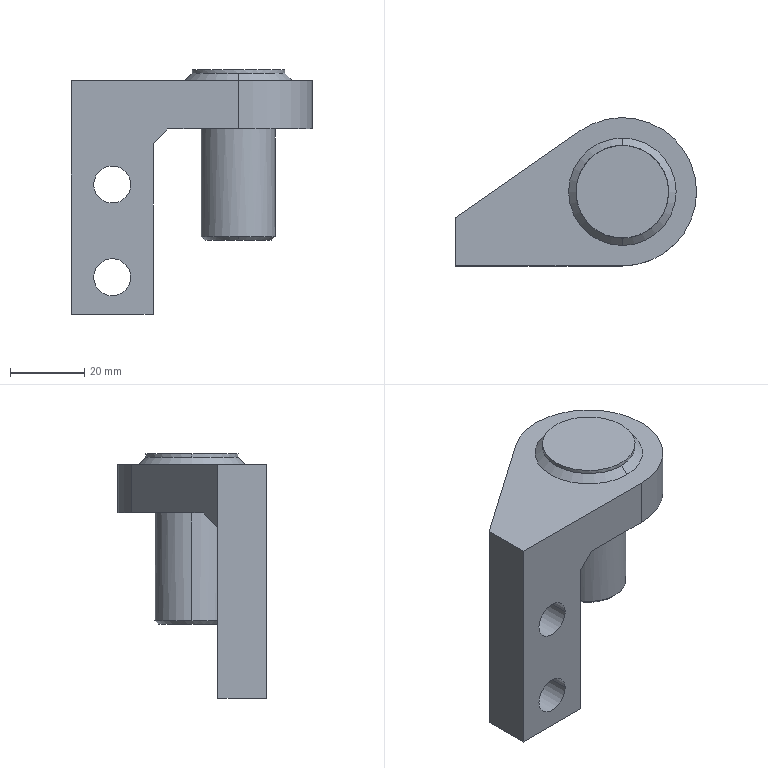Part | SolidWorks | features BaseBody 1 | 1 solid | 26 faces | box 65 x 40 x 66 mm | volume 48299 mm3 | plane 12 | cylinder 10 | cone 4 | commonest cylinder face diameters 10 x4 20 x2 25 x2 40 x2
STEP:
#1=CARTESIAN_POINT('',(14.621,16.327,0.));
#2=VERTEX_POINT('',#1);
#3=CARTESIAN_POINT('',(34.621,16.327,0.));
#4=VERTEX_POINT('',#3);
#5=CARTESIAN_POINT('',(24.621,16.327,0.));
#6=DIRECTION('',(0.,0.,-1.));
#7=DIRECTION('',(-1.,0.,0.));
#8=AXIS2_PLACEMENT_3D('',#5,#6,#7);
#9=CIRCLE('',#8,10.);
#10=EDGE_CURVE('',#2,#4,#9,.T.);
#11=ORIENTED_EDGE('',*,*,#10,.T.);
#12=CARTESIAN_POINT('',(34.621,16.327,-29.));
#13=VERTEX_POINT('',#12);
#14=CARTESIAN_POINT('',(34.621,16.327,0.));
#15=DIRECTION('',(0.,0.,-1.));
#16=VECTOR('',#15,1000.);
#17=LINE('',#14,#16);
#18=EDGE_CURVE('',#4,#13,#17,.T.);
#19=ORIENTED_EDGE('',*,*,#18,.T.);
#20=CARTESIAN_POINT('',(24.621,26.327,-29.));
#21=VERTEX_POINT('',#20);
#22=CARTESIAN_POINT('',(24.621,16.327,-29.));
#23=DIRECTION('',(0.,0.,1.));
#24=DIRECTION('',(-1.,0.,0.));
#25=AXIS2_PLACEMENT_3D('',#22,#23,#24);
#26=CIRCLE('',#25,10.);
#27=EDGE_CURVE('',#13,#21,#26,.T.);
#28=ORIENTED_EDGE('',*,*,#27,.T.);
#29=CARTESIAN_POINT('',(14.621,16.327,-29.));
#30=VERTEX_POINT('',#29);
#31=CARTESIAN_POINT('',(24.621,16.327,-29.));
#32=DIRECTION('',(0.,0.,1.));
#33=DIRECTION('',(-1.,0.,0.));
#34=AXIS2_PLACEMENT_3D('',#31,#32,#33);
#35=CIRCLE('',#34,10.);
#36=EDGE_CURVE('',#21,#30,#35,.T.);
#37=ORIENTED_EDGE('',*,*,#36,.T.);
#38=CARTESIAN_POINT('',(14.621,16.327,0.));
#39=DIRECTION('',(0.,0.,-1.));
#40=VECTOR('',#39,1000.);
#41=LINE('',#38,#40);
#42=EDGE_CURVE('',#2,#30,#41,.T.);
#43=ORIENTED_EDGE('',*,*,#42,.F.);
#44=EDGE_LOOP('',(#11,#19,#28,#37,#43));
#45=FACE_OUTER_BOUND('',#44,.T.);
#46=CARTESIAN_POINT('',(24.621,16.327,0.));
#47=DIRECTION('',(0.,0.,-1.));
#48=DIRECTION('',(-1.,0.,0.));
#49=AXIS2_PLACEMENT_3D('',#46,#47,#48);
#50=CYLINDRICAL_SURFACE('',#49,10.);
#51=ADVANCED_FACE('',(#45),#50,.T.);
#52=CARTESIAN_POINT('',(24.621,7.327,-30.));
#53=VERTEX_POINT('',#52);
#54=CARTESIAN_POINT('',(24.621,25.327,-30.));
#55=VERTEX_POINT('',#54);
#56=CARTESIAN_POINT('',(24.621,16.327,-30.));
#57=DIRECTION('',(0.,0.,1.));
#58=DIRECTION('',(0.,-1.,0.));
#59=AXIS2_PLACEMENT_3D('',#56,#57,#58);
#60=CIRCLE('',#59,9.);
#61=EDGE_CURVE('',#53,#55,#60,.T.);
#62=ORIENTED_EDGE('',*,*,#61,.T.);
#63=CARTESIAN_POINT('',(24.621,26.327,-29.));
#64=DIRECTION('',(0.,0.7071,0.7071));
#65=VECTOR('',#64,1000.);
#66=LINE('',#63,#65);
#67=EDGE_CURVE('',#55,#21,#66,.T.);
#68=ORIENTED_EDGE('',*,*,#67,.T.);
#69=ORIENTED_EDGE('',*,*,#27,.F.);
#70=CARTESIAN_POINT('',(24.621,6.327,-29.));
#71=VERTEX_POINT('',#70);
#72=CARTESIAN_POINT('',(24.621,16.327,-29.));
#73=DIRECTION('',(0.,0.,1.));
#74=DIRECTION('',(-1.,0.,0.));
#75=AXIS2_PLACEMENT_3D('',#72,#73,#74);
#76=CIRCLE('',#75,10.);
#77=EDGE_CURVE('',#71,#13,#76,.T.);
#78=ORIENTED_EDGE('',*,*,#77,.F.);
#79=CARTESIAN_POINT('',(24.621,6.327,-29.));
#80=DIRECTION('',(0.,-0.7071,0.7071));
#81=VECTOR('',#80,1000.);
#82=LINE('',#79,#81);
#83=EDGE_CURVE('',#53,#71,#82,.T.);
#84=ORIENTED_EDGE('',*,*,#83,.F.);
#85=EDGE_LOOP('',(#62,#68,#69,#78,#84));
#86=FACE_OUTER_BOUND('',#85,.T.);
#87=CARTESIAN_POINT('',(24.621,16.327,-29.));
#88=DIRECTION('',(0.,0.,1.));
#89=DIRECTION('',(0.,-1.,0.));
#90=AXIS2_PLACEMENT_3D('',#87,#88,#89);
#91=CONICAL_SURFACE('',#90,10.,0.7854);
#92=ADVANCED_FACE('',(#86),#91,.T.);
#93=CARTESIAN_POINT('',(24.621,-3.673,0.));
#94=VERTEX_POINT('',#93);
#95=CARTESIAN_POINT('',(44.621,16.327,0.));
#96=VERTEX_POINT('',#95);
#97=CARTESIAN_POINT('',(24.621,16.327,0.));
#98=DIRECTION('',(0.,0.,1.));
#99=DIRECTION('',(1.,0.,0.));
#100=AXIS2_PLACEMENT_3D('',#97,#98,#99);
#101=CIRCLE('',#100,20.);
#102=EDGE_CURVE('',#94,#96,#101,.T.);
#103=ORIENTED_EDGE('',*,*,#102,.T.);
#104=CARTESIAN_POINT('',(44.621,16.327,13.));
#105=VERTEX_POINT('',#104);
#106=CARTESIAN_POINT('',(44.621,16.327,0.));
#107=DIRECTION('',(0.,0.,1.));
#108=VECTOR('',#107,1000.);
#109=LINE('',#106,#108);
#110=EDGE_CURVE('',#96,#105,#109,.T.);
#111=ORIENTED_EDGE('',*,*,#110,.T.);
#112=CARTESIAN_POINT('',(24.621,-3.673,13.));
#113=VERTEX_POINT('',#112);
#114=CARTESIAN_POINT('',(24.621,16.327,13.));
#115=DIRECTION('',(0.,0.,-1.));
#116=DIRECTION('',(1.,0.,0.));
#117=AXIS2_PLACEMENT_3D('',#114,#115,#116);
#118=CIRCLE('',#117,20.);
#119=EDGE_CURVE('',#105,#113,#118,.T.);
#120=ORIENTED_EDGE('',*,*,#119,.T.);
#121=CARTESIAN_POINT('',(24.621,-3.673,0.));
#122=DIRECTION('',(0.,0.,-1.));
#123=VECTOR('',#122,1000.);
#124=LINE('',#121,#123);
#125=EDGE_CURVE('',#113,#94,#124,.T.);
#126=ORIENTED_EDGE('',*,*,#125,.T.);
#127=EDGE_LOOP('',(#103,#111,#120,#126));
#128=FACE_OUTER_BOUND('',#127,.T.);
#129=CARTESIAN_POINT('',(24.621,16.327,0.));
#130=DIRECTION('',(0.,0.,1.));
#131=DIRECTION('',(1.,0.,0.));
#132=AXIS2_PLACEMENT_3D('',#129,#130,#131);
#133=CYLINDRICAL_SURFACE('',#132,20.);
#134=ADVANCED_FACE('',(#128),#133,.T.);
#135=CARTESIAN_POINT('',(-4.379,-3.673,-40.));
#136=VERTEX_POINT('',#135);
#137=CARTESIAN_POINT('',(-14.379,-3.673,-40.));
#138=VERTEX_POINT('',#137);
#139=CARTESIAN_POINT('',(-9.379,-3.673,-40.));
#140=DIRECTION('',(0.,1.,0.));
#141=DIRECTION('',(-1.,0.,0.));
#142=AXIS2_PLACEMENT_3D('',#139,#140,#141);
#143=CIRCLE('',#142,5.);
#144=EDGE_CURVE('',#136,#138,#143,.T.);
#145=ORIENTED_EDGE('',*,*,#144,.F.);
#146=CARTESIAN_POINT('',(-4.379,9.327,-40.));
#147=VERTEX_POINT('',#146);
#148=CARTESIAN_POINT('',(-4.379,-91.574,-40.));
#149=DIRECTION('',(0.,1.,0.));
#150=VECTOR('',#149,1000.);
#151=LINE('',#148,#150);
#152=EDGE_CURVE('',#136,#147,#151,.T.);
#153=ORIENTED_EDGE('',*,*,#152,.T.);
#154=CARTESIAN_POINT('',(-14.379,9.327,-40.));
#155=VERTEX_POINT('',#154);
#156=CARTESIAN_POINT('',(-9.379,9.327,-40.));
#157=DIRECTION('',(0.,-1.,0.));
#158=DIRECTION('',(-1.,0.,0.));
#159=AXIS2_PLACEMENT_3D('',#156,#157,#158);
#160=CIRCLE('',#159,5.);
#161=EDGE_CURVE('',#155,#147,#160,.T.);
#162=ORIENTED_EDGE('',*,*,#161,.F.);
#163=CARTESIAN_POINT('',(-14.379,-91.574,-40.));
#164=DIRECTION('',(0.,1.,0.));
#165=VECTOR('',#164,1000.);
#166=LINE('',#163,#165);
#167=EDGE_CURVE('',#138,#155,#166,.T.);
#168=ORIENTED_EDGE('',*,*,#167,.F.);
#169=EDGE_LOOP('',(#145,#153,#162,#168));
#170=FACE_OUTER_BOUND('',#169,.T.);
#171=CARTESIAN_POINT('',(-9.379,-91.574,-40.));
#172=DIRECTION('',(0.,1.,0.));
#173=DIRECTION('',(-1.,0.,0.));
#174=AXIS2_PLACEMENT_3D('',#171,#172,#173);
#175=CYLINDRICAL_SURFACE('',#174,5.);
#176=ADVANCED_FACE('',(#170),#175,.F.);
#177=CARTESIAN_POINT('',(-4.379,-3.673,-15.));
#178=VERTEX_POINT('',#177);
#179=CARTESIAN_POINT('',(-14.379,-3.673,-15.));
#180=VERTEX_POINT('',#179);
#181=CARTESIAN_POINT('',(-9.379,-3.673,-15.));
#182=DIRECTION('',(0.,1.,0.));
#183=DIRECTION('',(-1.,0.,0.));
#184=AXIS2_PLACEMENT_3D('',#181,#182,#183);
#185=CIRCLE('',#184,5.);
#186=EDGE_CURVE('',#178,#180,#185,.T.);
#187=ORIENTED_EDGE('',*,*,#186,.F.);
#188=CARTESIAN_POINT('',(-4.379,9.327,-15.));
#189=VERTEX_POINT('',#188);
#190=CARTESIAN_POINT('',(-4.379,-91.574,-15.));
#191=DIRECTION('',(0.,1.,0.));
#192=VECTOR('',#191,1000.);
#193=LINE('',#190,#192);
#194=EDGE_CURVE('',#178,#189,#193,.T.);
#195=ORIENTED_EDGE('',*,*,#194,.T.);
#196=CARTESIAN_POINT('',(-14.379,9.327,-15.));
#197=VERTEX_POINT('',#196);
#198=CARTESIAN_POINT('',(-9.379,9.327,-15.));
#199=DIRECTION('',(0.,-1.,0.));
#200=DIRECTION('',(-1.,0.,0.));
#201=AXIS2_PLACEMENT_3D('',#198,#199,#200);
#202=CIRCLE('',#201,5.);
#203=EDGE_CURVE('',#197,#189,#202,.T.);
#204=ORIENTED_EDGE('',*,*,#203,.F.);
#205=CARTESIAN_POINT('',(-14.379,-91.574,-15.));
#206=DIRECTION('',(0.,1.,0.));
#207=VECTOR('',#206,1000.);
#208=LINE('',#205,#207);
#209=EDGE_CURVE('',#180,#197,#208,.T.);
#210=ORIENTED_EDGE('',*,*,#209,.F.);
#211=EDGE_LOOP('',(#187,#195,#204,#210));
#212=FACE_OUTER_BOUND('',#211,.T.);
#213=CARTESIAN_POINT('',(-9.379,-91.574,-15.));
#214=DIRECTION('',(0.,1.,0.));
#215=DIRECTION('',(-1.,0.,0.));
#216=AXIS2_PLACEMENT_3D('',#213,#214,#215);
#217=CYLINDRICAL_SURFACE('',#216,5.);
#218=ADVANCED_FACE('',(#212),#217,.F.);
#219=CARTESIAN_POINT('',(37.121,16.327,15.));
#220=VERTEX_POINT('',#219);
#221=CARTESIAN_POINT('',(24.621,3.827,15.));
#222=VERTEX_POINT('',#221);
#223=CARTESIAN_POINT('',(24.621,16.327,15.));
#224=DIRECTION('',(0.,0.,-1.));
#225=DIRECTION('',(-1.,0.,0.));
#226=AXIS2_PLACEMENT_3D('',#223,#224,#225);
#227=CIRCLE('',#226,12.5);
#228=EDGE_CURVE('',#220,#222,#227,.T.);
#229=ORIENTED_EDGE('',*,*,#228,.T.);
#230=CARTESIAN_POINT('',(24.621,1.827,13.));
#231=VERTEX_POINT('',#230);
#232=CARTESIAN_POINT('',(24.621,1.827,13.));
#233=DIRECTION('',(0.,-0.7071,-0.7071));
#234=VECTOR('',#233,1000.);
#235=LINE('',#232,#234);
#236=EDGE_CURVE('',#222,#231,#235,.T.);
#237=ORIENTED_EDGE('',*,*,#236,.T.);
#238=CARTESIAN_POINT('',(24.621,30.827,13.));
#239=VERTEX_POINT('',#238);
#240=CARTESIAN_POINT('',(24.621,16.327,13.));
#241=DIRECTION('',(0.,0.,-1.));
#242=DIRECTION('',(0.,1.,0.));
#243=AXIS2_PLACEMENT_3D('',#240,#241,#242);
#244=CIRCLE('',#243,14.5);
#245=EDGE_CURVE('',#239,#231,#244,.T.);
#246=ORIENTED_EDGE('',*,*,#245,.F.);
#247=CARTESIAN_POINT('',(24.621,28.827,15.));
#248=VERTEX_POINT('',#247);
#249=CARTESIAN_POINT('',(24.621,30.827,13.));
#250=DIRECTION('',(0.,0.7071,-0.7071));
#251=VECTOR('',#250,1000.);
#252=LINE('',#249,#251);
#253=EDGE_CURVE('',#248,#239,#252,.T.);
#254=ORIENTED_EDGE('',*,*,#253,.F.);
#255=CARTESIAN_POINT('',(24.621,16.327,15.));
#256=DIRECTION('',(0.,0.,-1.));
#257=DIRECTION('',(-1.,0.,0.));
#258=AXIS2_PLACEMENT_3D('',#255,#256,#257);
#259=CIRCLE('',#258,12.5);
#260=EDGE_CURVE('',#248,#220,#259,.T.);
#261=ORIENTED_EDGE('',*,*,#260,.T.);
#262=EDGE_LOOP('',(#229,#237,#246,#254,#261));
#263=FACE_OUTER_BOUND('',#262,.T.);
#264=CARTESIAN_POINT('',(24.621,16.327,13.));
#265=DIRECTION('',(0.,0.,-1.));
#266=DIRECTION('',(0.,1.,0.));
#267=AXIS2_PLACEMENT_3D('',#264,#265,#266);
#268=CONICAL_SURFACE('',#267,14.5,0.7854);
#269=ADVANCED_FACE('',(#263),#268,.T.);
#270=CARTESIAN_POINT('',(12.121,16.327,15.));
#271=VERTEX_POINT('',#270);
#272=CARTESIAN_POINT('',(24.621,16.327,15.));
#273=DIRECTION('',(0.,0.,-1.));
#274=DIRECTION('',(-1.,0.,0.));
#275=AXIS2_PLACEMENT_3D('',#272,#273,#274);
#276=CIRCLE('',#275,12.5);
#277=EDGE_CURVE('',#271,#248,#276,.T.);
#278=ORIENTED_EDGE('',*,*,#277,.F.);
#279=CARTESIAN_POINT('',(12.121,16.327,16.));
#280=VERTEX_POINT('',#279);
#281=CARTESIAN_POINT('',(12.121,16.327,13.));
#282=DIRECTION('',(0.,0.,1.));
#283=VECTOR('',#282,1000.);
#284=LINE('',#281,#283);
#285=EDGE_CURVE('',#271,#280,#284,.T.);
#286=ORIENTED_EDGE('',*,*,#285,.T.);
#287=CARTESIAN_POINT('',(37.121,16.327,16.));
#288=VERTEX_POINT('',#287);
#289=CARTESIAN_POINT('',(24.621,16.327,16.));
#290=DIRECTION('',(0.,0.,-1.));
#291=DIRECTION('',(1.,0.,0.));
#292=AXIS2_PLACEMENT_3D('',#289,#290,#291);
#293=CIRCLE('',#292,12.5);
#294=EDGE_CURVE('',#280,#288,#293,.T.);
#295=ORIENTED_EDGE('',*,*,#294,.T.);
#296=CARTESIAN_POINT('',(37.121,16.327,13.));
#297=DIRECTION('',(0.,0.,1.));
#298=VECTOR('',#297,1000.);
#299=LINE('',#296,#298);
#300=EDGE_CURVE('',#220,#288,#299,.T.);
#301=ORIENTED_EDGE('',*,*,#300,.F.);
#302=ORIENTED_EDGE('',*,*,#260,.F.);
#303=EDGE_LOOP('',(#278,#286,#295,#301,#302));
#304=FACE_OUTER_BOUND('',#303,.T.);
#305=CARTESIAN_POINT('',(24.621,16.327,13.));
#306=DIRECTION('',(0.,0.,1.));
#307=DIRECTION('',(1.,0.,0.));
#308=AXIS2_PLACEMENT_3D('',#305,#306,#307);
#309=CYLINDRICAL_SURFACE('',#308,12.5);
#310=ADVANCED_FACE('',(#304),#309,.T.);
#311=ORIENTED_EDGE('',*,*,#18,.F.);
#312=CARTESIAN_POINT('',(24.621,16.327,0.));
#313=DIRECTION('',(0.,0.,-1.));
#314=DIRECTION('',(-1.,0.,0.));
#315=AXIS2_PLACEMENT_3D('',#312,#313,#314);
#316=CIRCLE('',#315,10.);
#317=EDGE_CURVE('',#4,#2,#316,.T.);
#318=ORIENTED_EDGE('',*,*,#317,.T.);
#319=ORIENTED_EDGE('',*,*,#42,.T.);
#320=CARTESIAN_POINT('',(24.621,16.327,-29.));
#321=DIRECTION('',(0.,0.,1.));
#322=DIRECTION('',(-1.,0.,0.));
#323=AXIS2_PLACEMENT_3D('',#320,#321,#322);
#324=CIRCLE('',#323,10.);
#325=EDGE_CURVE('',#30,#71,#324,.T.);
#326=ORIENTED_EDGE('',*,*,#325,.T.);
#327=ORIENTED_EDGE('',*,*,#77,.T.);
#328=EDGE_LOOP('',(#311,#318,#319,#326,#327));
#329=FACE_OUTER_BOUND('',#328,.T.);
#330=CARTESIAN_POINT('',(24.621,16.327,0.));
#331=DIRECTION('',(0.,0.,-1.));
#332=DIRECTION('',(-1.,0.,0.));
#333=AXIS2_PLACEMENT_3D('',#330,#331,#332);
#334=CYLINDRICAL_SURFACE('',#333,10.);
#335=ADVANCED_FACE('',(#329),#334,.T.);
#336=ORIENTED_EDGE('',*,*,#67,.F.);
#337=CARTESIAN_POINT('',(24.621,16.327,-30.));
#338=DIRECTION('',(0.,0.,1.));
#339=DIRECTION('',(0.,-1.,0.));
#340=AXIS2_PLACEMENT_3D('',#337,#338,#339);
#341=CIRCLE('',#340,9.);
#342=EDGE_CURVE('',#55,#53,#341,.T.);
#343=ORIENTED_EDGE('',*,*,#342,.T.);
#344=ORIENTED_EDGE('',*,*,#83,.T.);
#345=ORIENTED_EDGE('',*,*,#325,.F.);
#346=ORIENTED_EDGE('',*,*,#36,.F.);
#347=EDGE_LOOP('',(#336,#343,#344,#345,#346));
#348=FACE_OUTER_BOUND('',#347,.T.);
#349=CARTESIAN_POINT('',(24.621,16.327,-29.));
#350=DIRECTION('',(0.,0.,1.));
#351=DIRECTION('',(0.,-1.,0.));
#352=AXIS2_PLACEMENT_3D('',#349,#350,#351);
#353=CONICAL_SURFACE('',#352,10.,0.7854);
#354=ADVANCED_FACE('',(#348),#353,.T.);
#355=ORIENTED_EDGE('',*,*,#10,.F.);
#356=ORIENTED_EDGE('',*,*,#317,.F.);
#357=EDGE_LOOP('',(#355,#356));
#358=FACE_BOUND('',#357,.T.);
#359=CARTESIAN_POINT('',(-14.644,13.327,0.));
#360=VERTEX_POINT('',#359);
#361=CARTESIAN_POINT('',(5.621,13.327,0.));
#362=VERTEX_POINT('',#361);
#363=CARTESIAN_POINT('',(12.334,13.327,0.));
#364=DIRECTION('',(1.,0.,0.));
#365=VECTOR('',#364,1000.);
#366=LINE('',#363,#365);
#367=EDGE_CURVE('',#360,#362,#366,.T.);
#368=ORIENTED_EDGE('',*,*,#367,.F.);
#369=CARTESIAN_POINT('',(13.18,32.732,0.));
#370=VERTEX_POINT('',#369);
#371=CARTESIAN_POINT('',(13.18,32.732,0.));
#372=DIRECTION('',(-0.8202,-0.572,0.));
#373=VECTOR('',#372,1000.);
#374=LINE('',#371,#373);
#375=EDGE_CURVE('',#370,#360,#374,.T.);
#376=ORIENTED_EDGE('',*,*,#375,.F.);
#377=CARTESIAN_POINT('',(24.621,16.327,0.));
#378=DIRECTION('',(0.,0.,1.));
#379=DIRECTION('',(1.,0.,0.));
#380=AXIS2_PLACEMENT_3D('',#377,#378,#379);
#381=CIRCLE('',#380,20.);
#382=EDGE_CURVE('',#96,#370,#381,.T.);
#383=ORIENTED_EDGE('',*,*,#382,.F.);
#384=ORIENTED_EDGE('',*,*,#102,.F.);
#385=CARTESIAN_POINT('',(5.621,-3.673,0.));
#386=VERTEX_POINT('',#385);
#387=CARTESIAN_POINT('',(12.334,-3.673,0.));
#388=DIRECTION('',(1.,0.,0.));
#389=VECTOR('',#388,1000.);
#390=LINE('',#387,#389);
#391=EDGE_CURVE('',#386,#94,#390,.T.);
#392=ORIENTED_EDGE('',*,*,#391,.F.);
#393=CARTESIAN_POINT('',(5.621,12.361,0.));
#394=DIRECTION('',(0.,-1.,0.));
#395=VECTOR('',#394,1000.);
#396=LINE('',#393,#395);
#397=EDGE_CURVE('',#362,#386,#396,.T.);
#398=ORIENTED_EDGE('',*,*,#397,.F.);
#399=EDGE_LOOP('',(#368,#376,#383,#384,#392,#398));
#400=FACE_OUTER_BOUND('',#399,.T.);
#401=CARTESIAN_POINT('',(12.334,12.361,0.));
#402=DIRECTION('',(0.,0.,1.));
#403=DIRECTION('',(1.,0.,0.));
#404=AXIS2_PLACEMENT_3D('',#401,#402,#403);
#405=PLANE('',#404);
#406=ADVANCED_FACE('',(#358,#400),#405,.F.);
#407=ORIENTED_EDGE('',*,*,#61,.F.);
#408=ORIENTED_EDGE('',*,*,#342,.F.);
#409=EDGE_LOOP('',(#407,#408));
#410=FACE_OUTER_BOUND('',#409,.T.);
#411=CARTESIAN_POINT('',(24.621,16.327,-30.));
#412=DIRECTION('',(0.,0.,1.));
#413=DIRECTION('',(1.,0.,0.));
#414=AXIS2_PLACEMENT_3D('',#411,#412,#413);
#415=PLANE('',#414);
#416=ADVANCED_FACE('',(#410),#415,.F.);
#417=CARTESIAN_POINT('',(1.621,9.327,-4.));
#418=VERTEX_POINT('',#417);
#419=CARTESIAN_POINT('',(1.621,9.327,-4.));
#420=DIRECTION('',(0.5774,0.5774,0.5774));
#421=VECTOR('',#420,1000.);
#422=LINE('',#419,#421);
#423=EDGE_CURVE('',#418,#362,#422,.T.);
#424=ORIENTED_EDGE('',*,*,#423,.T.);
#425=ORIENTED_EDGE('',*,*,#397,.T.);
#426=CARTESIAN_POINT('',(1.621,-3.673,-4.));
#427=VERTEX_POINT('',#426);
#428=CARTESIAN_POINT('',(3.621,-3.673,-2.));
#429=DIRECTION('',(-0.7071,0.,-0.7071));
#430=VECTOR('',#429,1000.);
#431=LINE('',#428,#430);
#432=EDGE_CURVE('',#386,#427,#431,.T.);
#433=ORIENTED_EDGE('',*,*,#432,.T.);
#434=CARTESIAN_POINT('',(1.621,4.344,-4.));
#435=DIRECTION('',(0.,1.,0.));
#436=VECTOR('',#435,1000.);
#437=LINE('',#434,#436);
#438=EDGE_CURVE('',#427,#418,#437,.T.);
#439=ORIENTED_EDGE('',*,*,#438,.T.);
#440=EDGE_LOOP('',(#424,#425,#433,#439));
#441=FACE_OUTER_BOUND('',#440,.T.);
#442=CARTESIAN_POINT('',(3.621,4.344,-2.));
#443=DIRECTION('',(0.7071,0.,-0.7071));
#444=DIRECTION('',(-0.7071,0.,-0.7071));
#445=AXIS2_PLACEMENT_3D('',#442,#443,#444);
#446=PLANE('',#445);
#447=ADVANCED_FACE('',(#441),#446,.T.);
#448=ORIENTED_EDGE('',*,*,#423,.F.);
#449=CARTESIAN_POINT('',(-20.379,9.327,-4.));
#450=VERTEX_POINT('',#449);
#451=CARTESIAN_POINT('',(6.977,9.327,-4.));
#452=DIRECTION('',(-1.,0.,0.));
#453=VECTOR('',#452,1000.);
#454=LINE('',#451,#453);
#455=EDGE_CURVE('',#418,#450,#454,.T.);
#456=ORIENTED_EDGE('',*,*,#455,.T.);
#457=CARTESIAN_POINT('',(-20.379,9.327,-4.));
#458=DIRECTION('',(0.712,0.4965,0.4965));
#459=VECTOR('',#458,1000.);
#460=LINE('',#457,#459);
#461=EDGE_CURVE('',#450,#360,#460,.T.);
#462=ORIENTED_EDGE('',*,*,#461,.T.);
#463=ORIENTED_EDGE('',*,*,#367,.T.);
#464=EDGE_LOOP('',(#448,#456,#462,#463));
#465=FACE_OUTER_BOUND('',#464,.T.);
#466=CARTESIAN_POINT('',(6.977,11.327,-2.));
#467=DIRECTION('',(0.,0.7071,-0.7071));
#468=DIRECTION('',(0.,0.7071,0.7071));
#469=AXIS2_PLACEMENT_3D('',#466,#467,#468);
#470=PLANE('',#469);
#471=ADVANCED_FACE('',(#465),#470,.T.);
#472=ORIENTED_EDGE('',*,*,#461,.F.);
#473=CARTESIAN_POINT('',(-20.379,9.327,13.));
#474=VERTEX_POINT('',#473);
#475=CARTESIAN_POINT('',(-20.379,9.327,0.));
#476=DIRECTION('',(0.,0.,1.));
#477=VECTOR('',#476,1000.);
#478=LINE('',#475,#477);
#479=EDGE_CURVE('',#450,#474,#478,.T.);
#480=ORIENTED_EDGE('',*,*,#479,.T.);
#481=CARTESIAN_POINT('',(13.18,32.732,13.));
#482=VERTEX_POINT('',#481);
#483=CARTESIAN_POINT('',(-20.379,9.327,13.));
#484=DIRECTION('',(0.8202,0.572,0.));
#485=VECTOR('',#484,1000.);
#486=LINE('',#483,#485);
#487=EDGE_CURVE('',#474,#482,#486,.T.);
#488=ORIENTED_EDGE('',*,*,#487,.T.);
#489=CARTESIAN_POINT('',(13.18,32.732,0.));
#490=DIRECTION('',(0.,0.,-1.));
#491=VECTOR('',#490,1000.);
#492=LINE('',#489,#491);
#493=EDGE_CURVE('',#482,#370,#492,.T.);
#494=ORIENTED_EDGE('',*,*,#493,.T.);
#495=ORIENTED_EDGE('',*,*,#375,.T.);
#496=EDGE_LOOP('',(#472,#480,#488,#494,#495));
#497=FACE_OUTER_BOUND('',#496,.T.);
#498=CARTESIAN_POINT('',(-20.379,9.327,0.));
#499=DIRECTION('',(-0.572,0.8202,0.));
#500=DIRECTION('',(-0.8202,-0.572,0.));
#501=AXIS2_PLACEMENT_3D('',#498,#499,#500);
#502=PLANE('',#501);
#503=ADVANCED_FACE('',(#497),#502,.T.);
#504=ORIENTED_EDGE('',*,*,#110,.F.);
#505=ORIENTED_EDGE('',*,*,#382,.T.);
#506=ORIENTED_EDGE('',*,*,#493,.F.);
#507=CARTESIAN_POINT('',(24.621,16.327,13.));
#508=DIRECTION('',(0.,0.,-1.));
#509=DIRECTION('',(1.,0.,0.));
#510=AXIS2_PLACEMENT_3D('',#507,#508,#509);
#511=CIRCLE('',#510,20.);
#512=EDGE_CURVE('',#482,#105,#511,.T.);
#513=ORIENTED_EDGE('',*,*,#512,.T.);
#514=EDGE_LOOP('',(#504,#505,#506,#513));
#515=FACE_OUTER_BOUND('',#514,.T.);
#516=CARTESIAN_POINT('',(24.621,16.327,0.));
#517=DIRECTION('',(0.,0.,1.));
#518=DIRECTION('',(1.,0.,0.));
#519=AXIS2_PLACEMENT_3D('',#516,#517,#518);
#520=CYLINDRICAL_SURFACE('',#519,20.);
#521=ADVANCED_FACE('',(#515),#520,.T.);
#522=CARTESIAN_POINT('',(-9.379,-3.673,-40.));
#523=DIRECTION('',(0.,1.,0.));
#524=DIRECTION('',(-1.,0.,0.));
#525=AXIS2_PLACEMENT_3D('',#522,#523,#524);
#526=CIRCLE('',#525,5.);
#527=EDGE_CURVE('',#138,#136,#526,.T.);
#528=ORIENTED_EDGE('',*,*,#527,.T.);
#529=ORIENTED_EDGE('',*,*,#144,.T.);
#530=EDGE_LOOP('',(#528,#529));
#531=FACE_BOUND('',#530,.T.);
#532=CARTESIAN_POINT('',(-9.379,-3.673,-15.));
#533=DIRECTION('',(0.,1.,0.));
#534=DIRECTION('',(-1.,0.,0.));
#535=AXIS2_PLACEMENT_3D('',#532,#533,#534);
#536=CIRCLE('',#535,5.);
#537=EDGE_CURVE('',#180,#178,#536,.T.);
#538=ORIENTED_EDGE('',*,*,#537,.T.);
#539=ORIENTED_EDGE('',*,*,#186,.T.);
#540=EDGE_LOOP('',(#538,#539));
#541=FACE_BOUND('',#540,.T.);
#542=ORIENTED_EDGE('',*,*,#391,.T.);
#543=ORIENTED_EDGE('',*,*,#125,.F.);
#544=CARTESIAN_POINT('',(-20.379,-3.673,13.));
#545=VERTEX_POINT('',#544);
#546=CARTESIAN_POINT('',(24.621,-3.673,13.));
#547=DIRECTION('',(-1.,0.,0.));
#548=VECTOR('',#547,1000.);
#549=LINE('',#546,#548);
#550=EDGE_CURVE('',#113,#545,#549,.T.);
#551=ORIENTED_EDGE('',*,*,#550,.T.);
#552=CARTESIAN_POINT('',(-20.379,-3.673,-50.));
#553=VERTEX_POINT('',#552);
#554=CARTESIAN_POINT('',(-20.379,-3.673,0.));
#555=DIRECTION('',(0.,0.,-1.));
#556=VECTOR('',#555,1000.);
#557=LINE('',#554,#556);
#558=EDGE_CURVE('',#545,#553,#557,.T.);
#559=ORIENTED_EDGE('',*,*,#558,.T.);
#560=CARTESIAN_POINT('',(1.621,-3.673,-50.));
#561=VERTEX_POINT('',#560);
#562=CARTESIAN_POINT('',(24.621,-3.673,-50.));
#563=DIRECTION('',(1.,0.,0.));
#564=VECTOR('',#563,1000.);
#565=LINE('',#562,#564);
#566=EDGE_CURVE('',#553,#561,#565,.T.);
#567=ORIENTED_EDGE('',*,*,#566,.T.);
#568=CARTESIAN_POINT('',(1.621,-3.673,0.));
#569=DIRECTION('',(0.,0.,1.));
#570=VECTOR('',#569,1000.);
#571=LINE('',#568,#570);
#572=EDGE_CURVE('',#561,#427,#571,.T.);
#573=ORIENTED_EDGE('',*,*,#572,.T.);
#574=ORIENTED_EDGE('',*,*,#432,.F.);
#575=EDGE_LOOP('',(#542,#543,#551,#559,#567,#573,#574));
#576=FACE_OUTER_BOUND('',#575,.T.);
#577=CARTESIAN_POINT('',(24.621,-3.673,0.));
#578=DIRECTION('',(0.,-1.,0.));
#579=DIRECTION('',(0.,0.,-1.));
#580=AXIS2_PLACEMENT_3D('',#577,#578,#579);
#581=PLANE('',#580);
#582=ADVANCED_FACE('',(#531,#541,#576),#581,.T.);
#583=CARTESIAN_POINT('',(1.621,9.327,-50.));
#584=VERTEX_POINT('',#583);
#585=CARTESIAN_POINT('',(1.621,-3.673,-50.));
#586=DIRECTION('',(0.,1.,0.));
#587=VECTOR('',#586,1000.);
#588=LINE('',#585,#587);
#589=EDGE_CURVE('',#561,#584,#588,.T.);
#590=ORIENTED_EDGE('',*,*,#589,.T.);
#591=CARTESIAN_POINT('',(1.621,9.327,0.));
#592=DIRECTION('',(0.,0.,1.));
#593=VECTOR('',#592,1000.);
#594=LINE('',#591,#593);
#595=EDGE_CURVE('',#584,#418,#594,.T.);
#596=ORIENTED_EDGE('',*,*,#595,.T.);
#597=ORIENTED_EDGE('',*,*,#438,.F.);
#598=ORIENTED_EDGE('',*,*,#572,.F.);
#599=EDGE_LOOP('',(#590,#596,#597,#598));
#600=FACE_OUTER_BOUND('',#599,.T.);
#601=CARTESIAN_POINT('',(1.621,-3.673,0.));
#602=DIRECTION('',(1.,0.,0.));
#603=DIRECTION('',(0.,1.,0.));
#604=AXIS2_PLACEMENT_3D('',#601,#602,#603);
#605=PLANE('',#604);
#606=ADVANCED_FACE('',(#600),#605,.T.);
#607=ORIENTED_EDGE('',*,*,#161,.T.);
#608=CARTESIAN_POINT('',(-9.379,9.327,-40.));
#609=DIRECTION('',(0.,-1.,0.));
#610=DIRECTION('',(-1.,0.,0.));
#611=AXIS2_PLACEMENT_3D('',#608,#609,#610);
#612=CIRCLE('',#611,5.);
#613=EDGE_CURVE('',#147,#155,#612,.T.);
#614=ORIENTED_EDGE('',*,*,#613,.T.);
#615=EDGE_LOOP('',(#607,#614));
#616=FACE_BOUND('',#615,.T.);
#617=ORIENTED_EDGE('',*,*,#203,.T.);
#618=CARTESIAN_POINT('',(-9.379,9.327,-15.));
#619=DIRECTION('',(0.,-1.,0.));
#620=DIRECTION('',(-1.,0.,0.));
#621=AXIS2_PLACEMENT_3D('',#618,#619,#620);
#622=CIRCLE('',#621,5.);
#623=EDGE_CURVE('',#189,#197,#622,.T.);
#624=ORIENTED_EDGE('',*,*,#623,.T.);
#625=EDGE_LOOP('',(#617,#624));
#626=FACE_BOUND('',#625,.T.);
#627=CARTESIAN_POINT('',(-20.379,9.327,-50.));
#628=VERTEX_POINT('',#627);
#629=CARTESIAN_POINT('',(1.621,9.327,-50.));
#630=DIRECTION('',(-1.,0.,0.));
#631=VECTOR('',#630,1000.);
#632=LINE('',#629,#631);
#633=EDGE_CURVE('',#584,#628,#632,.T.);
#634=ORIENTED_EDGE('',*,*,#633,.T.);
#635=CARTESIAN_POINT('',(-20.379,9.327,0.));
#636=DIRECTION('',(0.,0.,1.));
#637=VECTOR('',#636,1000.);
#638=LINE('',#635,#637);
#639=EDGE_CURVE('',#628,#450,#638,.T.);
#640=ORIENTED_EDGE('',*,*,#639,.T.);
#641=ORIENTED_EDGE('',*,*,#455,.F.);
#642=ORIENTED_EDGE('',*,*,#595,.F.);
#643=EDGE_LOOP('',(#634,#640,#641,#642));
#644=FACE_OUTER_BOUND('',#643,.T.);
#645=CARTESIAN_POINT('',(1.621,9.327,0.));
#646=DIRECTION('',(0.,1.,0.));
#647=DIRECTION('',(-1.,0.,0.));
#648=AXIS2_PLACEMENT_3D('',#645,#646,#647);
#649=PLANE('',#648);
#650=ADVANCED_FACE('',(#616,#626,#644),#649,.T.);
#651=CARTESIAN_POINT('',(-20.379,-3.673,-50.));
#652=DIRECTION('',(0.,-1.,0.));
#653=VECTOR('',#652,1000.);
#654=LINE('',#651,#653);
#655=EDGE_CURVE('',#628,#553,#654,.T.);
#656=ORIENTED_EDGE('',*,*,#655,.T.);
#657=ORIENTED_EDGE('',*,*,#558,.F.);
#658=CARTESIAN_POINT('',(-20.379,-3.673,13.));
#659=DIRECTION('',(0.,1.,0.));
#660=VECTOR('',#659,1000.);
#661=LINE('',#658,#660);
#662=EDGE_CURVE('',#545,#474,#661,.T.);
#663=ORIENTED_EDGE('',*,*,#662,.T.);
#664=ORIENTED_EDGE('',*,*,#479,.F.);
#665=ORIENTED_EDGE('',*,*,#639,.F.);
#666=EDGE_LOOP('',(#656,#657,#663,#664,#665));
#667=FACE_OUTER_BOUND('',#666,.T.);
#668=CARTESIAN_POINT('',(-20.379,-3.673,0.));
#669=DIRECTION('',(-1.,0.,0.));
#670=DIRECTION('',(0.,-1.,0.));
#671=AXIS2_PLACEMENT_3D('',#668,#669,#670);
#672=PLANE('',#671);
#673=ADVANCED_FACE('',(#667),#672,.T.);
#674=ORIENTED_EDGE('',*,*,#245,.T.);
#675=CARTESIAN_POINT('',(24.621,16.327,13.));
#676=DIRECTION('',(0.,0.,-1.));
#677=DIRECTION('',(0.,1.,0.));
#678=AXIS2_PLACEMENT_3D('',#675,#676,#677);
#679=CIRCLE('',#678,14.5);
#680=EDGE_CURVE('',#231,#239,#679,.T.);
#681=ORIENTED_EDGE('',*,*,#680,.T.);
#682=EDGE_LOOP('',(#674,#681));
#683=FACE_BOUND('',#682,.T.);
#684=ORIENTED_EDGE('',*,*,#487,.F.);
#685=ORIENTED_EDGE('',*,*,#662,.F.);
#686=ORIENTED_EDGE('',*,*,#550,.F.);
#687=ORIENTED_EDGE('',*,*,#119,.F.);
#688=ORIENTED_EDGE('',*,*,#512,.F.);
#689=EDGE_LOOP('',(#684,#685,#686,#687,#688));
#690=FACE_OUTER_BOUND('',#689,.T.);
#691=CARTESIAN_POINT('',(12.334,12.361,13.));
#692=DIRECTION('',(0.,0.,1.));
#693=DIRECTION('',(1.,0.,0.));
#694=AXIS2_PLACEMENT_3D('',#691,#692,#693);
#695=PLANE('',#694);
#696=ADVANCED_FACE('',(#683,#690),#695,.T.);
#697=ORIENTED_EDGE('',*,*,#152,.F.);
#698=ORIENTED_EDGE('',*,*,#527,.F.);
#699=ORIENTED_EDGE('',*,*,#167,.T.);
#700=ORIENTED_EDGE('',*,*,#613,.F.);
#701=EDGE_LOOP('',(#697,#698,#699,#700));
#702=FACE_OUTER_BOUND('',#701,.T.);
#703=CARTESIAN_POINT('',(-9.379,-91.574,-40.));
#704=DIRECTION('',(0.,1.,0.));
#705=DIRECTION('',(-1.,0.,0.));
#706=AXIS2_PLACEMENT_3D('',#703,#704,#705);
#707=CYLINDRICAL_SURFACE('',#706,5.);
#708=ADVANCED_FACE('',(#702),#707,.F.);
#709=ORIENTED_EDGE('',*,*,#194,.F.);
#710=ORIENTED_EDGE('',*,*,#537,.F.);
#711=ORIENTED_EDGE('',*,*,#209,.T.);
#712=ORIENTED_EDGE('',*,*,#623,.F.);
#713=EDGE_LOOP('',(#709,#710,#711,#712));
#714=FACE_OUTER_BOUND('',#713,.T.);
#715=CARTESIAN_POINT('',(-9.379,-91.574,-15.));
#716=DIRECTION('',(0.,1.,0.));
#717=DIRECTION('',(-1.,0.,0.));
#718=AXIS2_PLACEMENT_3D('',#715,#716,#717);
#719=CYLINDRICAL_SURFACE('',#718,5.);
#720=ADVANCED_FACE('',(#714),#719,.F.);
#721=ORIENTED_EDGE('',*,*,#655,.F.);
#722=ORIENTED_EDGE('',*,*,#633,.F.);
#723=ORIENTED_EDGE('',*,*,#589,.F.);
#724=ORIENTED_EDGE('',*,*,#566,.F.);
#725=EDGE_LOOP('',(#721,#722,#723,#724));
#726=FACE_OUTER_BOUND('',#725,.T.);
#727=CARTESIAN_POINT('',(-9.379,2.827,-50.));
#728=DIRECTION('',(0.,0.,1.));
#729=DIRECTION('',(1.,0.,0.));
#730=AXIS2_PLACEMENT_3D('',#727,#728,#729);
#731=PLANE('',#730);
#732=ADVANCED_FACE('',(#726),#731,.F.);
#733=ORIENTED_EDGE('',*,*,#236,.F.);
#734=CARTESIAN_POINT('',(24.621,16.327,15.));
#735=DIRECTION('',(0.,0.,-1.));
#736=DIRECTION('',(-1.,0.,0.));
#737=AXIS2_PLACEMENT_3D('',#734,#735,#736);
#738=CIRCLE('',#737,12.5);
#739=EDGE_CURVE('',#222,#271,#738,.T.);
#740=ORIENTED_EDGE('',*,*,#739,.T.);
#741=ORIENTED_EDGE('',*,*,#277,.T.);
#742=ORIENTED_EDGE('',*,*,#253,.T.);
#743=ORIENTED_EDGE('',*,*,#680,.F.);
#744=EDGE_LOOP('',(#733,#740,#741,#742,#743));
#745=FACE_OUTER_BOUND('',#744,.T.);
#746=CARTESIAN_POINT('',(24.621,16.327,13.));
#747=DIRECTION('',(0.,0.,-1.));
#748=DIRECTION('',(0.,1.,0.));
#749=AXIS2_PLACEMENT_3D('',#746,#747,#748);
#750=CONICAL_SURFACE('',#749,14.5,0.7854);
#751=ADVANCED_FACE('',(#745),#750,.T.);
#752=ORIENTED_EDGE('',*,*,#285,.F.);
#753=ORIENTED_EDGE('',*,*,#739,.F.);
#754=ORIENTED_EDGE('',*,*,#228,.F.);
#755=ORIENTED_EDGE('',*,*,#300,.T.);
#756=CARTESIAN_POINT('',(24.621,16.327,16.));
#757=DIRECTION('',(0.,0.,-1.));
#758=DIRECTION('',(1.,0.,0.));
#759=AXIS2_PLACEMENT_3D('',#756,#757,#758);
#760=CIRCLE('',#759,12.5);
#761=EDGE_CURVE('',#288,#280,#760,.T.);
#762=ORIENTED_EDGE('',*,*,#761,.T.);
#763=EDGE_LOOP('',(#752,#753,#754,#755,#762));
#764=FACE_OUTER_BOUND('',#763,.T.);
#765=CARTESIAN_POINT('',(24.621,16.327,13.));
#766=DIRECTION('',(0.,0.,1.));
#767=DIRECTION('',(1.,0.,0.));
#768=AXIS2_PLACEMENT_3D('',#765,#766,#767);
#769=CYLINDRICAL_SURFACE('',#768,12.5);
#770=ADVANCED_FACE('',(#764),#769,.T.);
#771=ORIENTED_EDGE('',*,*,#761,.F.);
#772=ORIENTED_EDGE('',*,*,#294,.F.);
#773=EDGE_LOOP('',(#771,#772));
#774=FACE_OUTER_BOUND('',#773,.T.);
#775=CARTESIAN_POINT('',(24.621,16.327,16.));
#776=DIRECTION('',(0.,0.,-1.));
#777=DIRECTION('',(-1.,0.,0.));
#778=AXIS2_PLACEMENT_3D('',#775,#776,#777);
#779=PLANE('',#778);
#780=ADVANCED_FACE('',(#774),#779,.F.);
#781=CLOSED_SHELL('',(#51,#92,#134,#176,#218,#269,#310,#335,#354,#406,#416,#447,#471,#503,#521,#582,#606,#650,#673,#696,#708,#720,#732,#751,#770,#780));
#782=MANIFOLD_SOLID_BREP('',#781);
#783=CARTESIAN_POINT('',(0.,0.,0.));
#784=DIRECTION('',(0.,0.,1.));
#785=DIRECTION('',(1.,0.,0.));
#786=AXIS2_PLACEMENT_3D('',#783,#784,#785);
#787=(LENGTH_UNIT()NAMED_UNIT(*)SI_UNIT(.MILLI.,.METRE.));
#788=UNCERTAINTY_MEASURE_WITH_UNIT(LENGTH_MEASURE(0.00001),#787,'','');
#789=(NAMED_UNIT(*)PLANE_ANGLE_UNIT()SI_UNIT($,.RADIAN.));
#790=(NAMED_UNIT(*)SI_UNIT($,.STERADIAN.)SOLID_ANGLE_UNIT());
#791=(GEOMETRIC_REPRESENTATION_CONTEXT(3)GLOBAL_UNCERTAINTY_ASSIGNED_CONTEXT((#788))GLOBAL_UNIT_ASSIGNED_CONTEXT((#787,#789,#790))REPRESENTATION_CONTEXT('',''));
#792=ADVANCED_BREP_SHAPE_REPRESENTATION('',(#782,#786),#791);